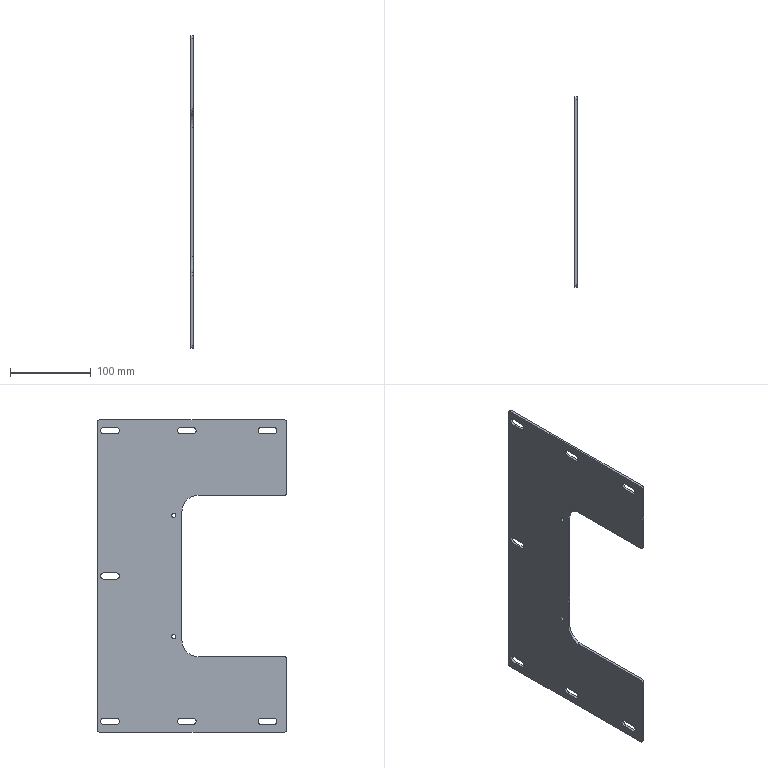Part | SolidWorks | features Fillet 3, FlatPattern 1, HoleWzd 1, ICE 1, SMBaseFlange 1, SheetMetal 1 | 1 solid | 50 faces | box 3 x 235 x 387 mm | volume 191622 mm3 | cylinder 26 | plane 24 | commonest cylinder face diameters 8 x14 6 x6 5 x4 40 x2